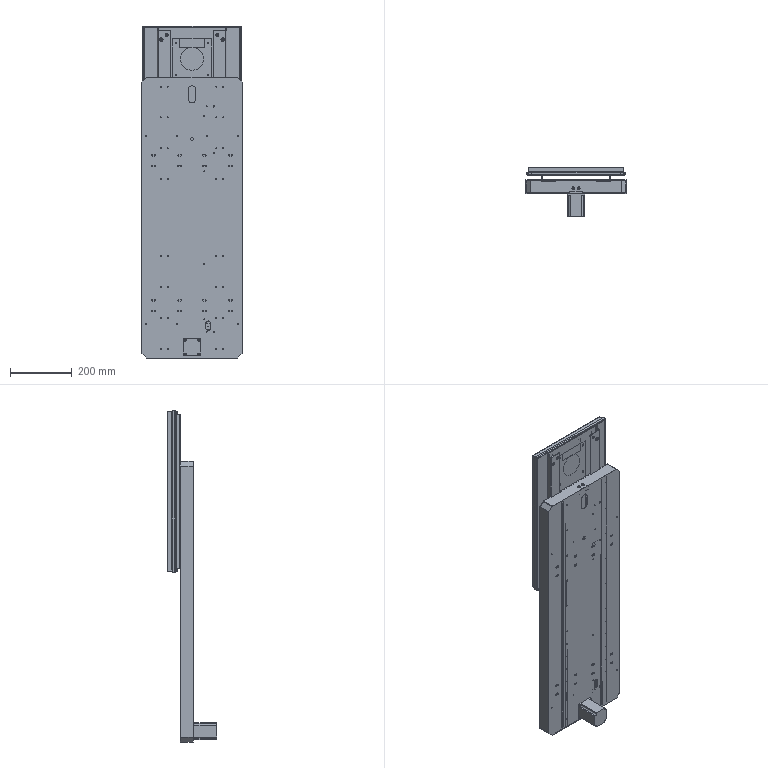Part | SolidWorks | 66 solids | 3968 faces | volume 5211065 mm3 | cylinder 2330 | plane 1041 | sphere 304 | torus 184 | cone 97 | spline 12 | commonest cylinder face diameters 1.5 x750 3.3 x178 0.56 x162 6 x150 0.3 x132 3.95 x126